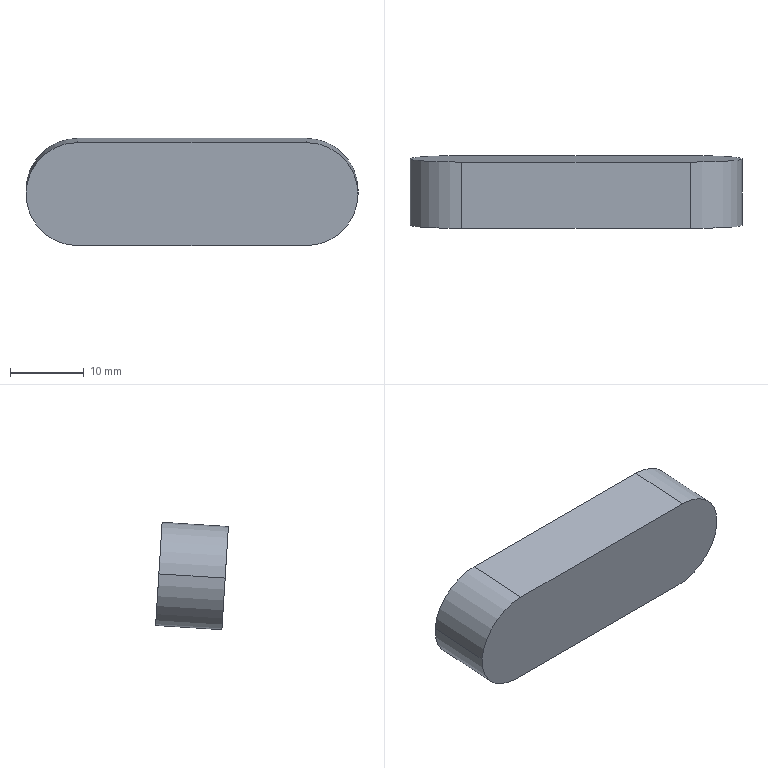Part | STEP file | Boss-Extrude 1-5 | 1 solid | 8 faces | box 45 x 9.869 x 14.542 mm | volume 5291 mm3 | cylinder 4 | plane 4 | commonest cylinder face diameters 14 x4
STEP:
#1=CARTESIAN_POINT('',(-140.476,-508.763,2440.556));
#2=VERTEX_POINT('',#1);
#3=CARTESIAN_POINT('',(-133.476,-509.206,2447.542));
#4=VERTEX_POINT('',#3);
#5=CARTESIAN_POINT('',(-133.476,-508.763,2440.556));
#6=DIRECTION('',(0.,0.998,0.06338));
#7=DIRECTION('',(-1.,0.,0.));
#8=AXIS2_PLACEMENT_3D('',#5,#6,#7);
#9=CIRCLE('',#8,7.);
#10=EDGE_CURVE('',#2,#4,#9,.T.);
#11=ORIENTED_EDGE('',*,*,#10,.F.);
#12=CARTESIAN_POINT('',(-140.476,-517.745,2439.986));
#13=VERTEX_POINT('',#12);
#14=CARTESIAN_POINT('',(-140.476,-508.763,2440.556));
#15=DIRECTION('',(0.,-0.998,-0.06338));
#16=VECTOR('',#15,1000.);
#17=LINE('',#14,#16);
#18=EDGE_CURVE('',#2,#13,#17,.T.);
#19=ORIENTED_EDGE('',*,*,#18,.T.);
#20=CARTESIAN_POINT('',(-133.476,-518.188,2446.972));
#21=VERTEX_POINT('',#20);
#22=CARTESIAN_POINT('',(-133.476,-517.745,2439.986));
#23=DIRECTION('',(0.,0.998,0.06338));
#24=DIRECTION('',(-1.,0.,0.));
#25=AXIS2_PLACEMENT_3D('',#22,#23,#24);
#26=CIRCLE('',#25,7.);
#27=EDGE_CURVE('',#13,#21,#26,.T.);
#28=ORIENTED_EDGE('',*,*,#27,.T.);
#29=CARTESIAN_POINT('',(-133.476,-509.206,2447.542));
#30=DIRECTION('',(0.,-0.998,-0.06338));
#31=VECTOR('',#30,1000.);
#32=LINE('',#29,#31);
#33=EDGE_CURVE('',#4,#21,#32,.T.);
#34=ORIENTED_EDGE('',*,*,#33,.F.);
#35=EDGE_LOOP('',(#11,#19,#28,#34));
#36=FACE_OUTER_BOUND('',#35,.T.);
#37=CARTESIAN_POINT('',(-133.476,-508.763,2440.556));
#38=DIRECTION('',(0.,-0.998,-0.06338));
#39=DIRECTION('',(-1.,0.,0.));
#40=AXIS2_PLACEMENT_3D('',#37,#38,#39);
#41=CYLINDRICAL_SURFACE('',#40,7.);
#42=ADVANCED_FACE('',(#36),#41,.T.);
#43=CARTESIAN_POINT('',(-95.476,-508.763,2440.556));
#44=VERTEX_POINT('',#43);
#45=CARTESIAN_POINT('',(-102.476,-508.319,2433.57));
#46=VERTEX_POINT('',#45);
#47=CARTESIAN_POINT('',(-102.476,-508.763,2440.556));
#48=DIRECTION('',(0.,0.998,0.06338));
#49=DIRECTION('',(-1.,0.,0.));
#50=AXIS2_PLACEMENT_3D('',#47,#48,#49);
#51=CIRCLE('',#50,7.);
#52=EDGE_CURVE('',#44,#46,#51,.T.);
#53=ORIENTED_EDGE('',*,*,#52,.F.);
#54=CARTESIAN_POINT('',(-95.476,-517.745,2439.986));
#55=VERTEX_POINT('',#54);
#56=CARTESIAN_POINT('',(-95.476,-508.763,2440.556));
#57=DIRECTION('',(0.,-0.998,-0.06338));
#58=VECTOR('',#57,1000.);
#59=LINE('',#56,#58);
#60=EDGE_CURVE('',#44,#55,#59,.T.);
#61=ORIENTED_EDGE('',*,*,#60,.T.);
#62=CARTESIAN_POINT('',(-102.476,-517.301,2433.));
#63=VERTEX_POINT('',#62);
#64=CARTESIAN_POINT('',(-102.476,-517.745,2439.986));
#65=DIRECTION('',(0.,0.998,0.06338));
#66=DIRECTION('',(-1.,0.,0.));
#67=AXIS2_PLACEMENT_3D('',#64,#65,#66);
#68=CIRCLE('',#67,7.);
#69=EDGE_CURVE('',#55,#63,#68,.T.);
#70=ORIENTED_EDGE('',*,*,#69,.T.);
#71=CARTESIAN_POINT('',(-102.476,-508.319,2433.57));
#72=DIRECTION('',(0.,-0.998,-0.06338));
#73=VECTOR('',#72,1000.);
#74=LINE('',#71,#73);
#75=EDGE_CURVE('',#46,#63,#74,.T.);
#76=ORIENTED_EDGE('',*,*,#75,.F.);
#77=EDGE_LOOP('',(#53,#61,#70,#76));
#78=FACE_OUTER_BOUND('',#77,.T.);
#79=CARTESIAN_POINT('',(-102.476,-508.763,2440.556));
#80=DIRECTION('',(0.,-0.998,-0.06338));
#81=DIRECTION('',(-1.,0.,0.));
#82=AXIS2_PLACEMENT_3D('',#79,#80,#81);
#83=CYLINDRICAL_SURFACE('',#82,7.);
#84=ADVANCED_FACE('',(#78),#83,.T.);
#85=ORIENTED_EDGE('',*,*,#60,.F.);
#86=CARTESIAN_POINT('',(-102.476,-509.206,2447.542));
#87=VERTEX_POINT('',#86);
#88=CARTESIAN_POINT('',(-102.476,-508.763,2440.556));
#89=DIRECTION('',(0.,0.998,0.06338));
#90=DIRECTION('',(-1.,0.,0.));
#91=AXIS2_PLACEMENT_3D('',#88,#89,#90);
#92=CIRCLE('',#91,7.);
#93=EDGE_CURVE('',#87,#44,#92,.T.);
#94=ORIENTED_EDGE('',*,*,#93,.F.);
#95=CARTESIAN_POINT('',(-102.476,-518.188,2446.972));
#96=VERTEX_POINT('',#95);
#97=CARTESIAN_POINT('',(-102.476,-509.206,2447.542));
#98=DIRECTION('',(0.,-0.998,-0.06338));
#99=VECTOR('',#98,1000.);
#100=LINE('',#97,#99);
#101=EDGE_CURVE('',#87,#96,#100,.T.);
#102=ORIENTED_EDGE('',*,*,#101,.T.);
#103=CARTESIAN_POINT('',(-102.476,-517.745,2439.986));
#104=DIRECTION('',(0.,0.998,0.06338));
#105=DIRECTION('',(-1.,0.,0.));
#106=AXIS2_PLACEMENT_3D('',#103,#104,#105);
#107=CIRCLE('',#106,7.);
#108=EDGE_CURVE('',#96,#55,#107,.T.);
#109=ORIENTED_EDGE('',*,*,#108,.T.);
#110=EDGE_LOOP('',(#85,#94,#102,#109));
#111=FACE_OUTER_BOUND('',#110,.T.);
#112=CARTESIAN_POINT('',(-102.476,-508.763,2440.556));
#113=DIRECTION('',(0.,-0.998,-0.06338));
#114=DIRECTION('',(-1.,0.,0.));
#115=AXIS2_PLACEMENT_3D('',#112,#113,#114);
#116=CYLINDRICAL_SURFACE('',#115,7.);
#117=ADVANCED_FACE('',(#111),#116,.T.);
#118=CARTESIAN_POINT('',(-133.476,-517.301,2433.));
#119=VERTEX_POINT('',#118);
#120=CARTESIAN_POINT('',(-102.476,-517.301,2433.));
#121=DIRECTION('',(-1.,0.,0.));
#122=VECTOR('',#121,1000.);
#123=LINE('',#120,#122);
#124=EDGE_CURVE('',#63,#119,#123,.T.);
#125=ORIENTED_EDGE('',*,*,#124,.T.);
#126=CARTESIAN_POINT('',(-133.476,-508.319,2433.57));
#127=VERTEX_POINT('',#126);
#128=CARTESIAN_POINT('',(-133.476,-508.319,2433.57));
#129=DIRECTION('',(0.,-0.998,-0.06338));
#130=VECTOR('',#129,1000.);
#131=LINE('',#128,#130);
#132=EDGE_CURVE('',#127,#119,#131,.T.);
#133=ORIENTED_EDGE('',*,*,#132,.F.);
#134=CARTESIAN_POINT('',(-102.476,-508.319,2433.57));
#135=DIRECTION('',(-1.,0.,0.));
#136=VECTOR('',#135,1000.);
#137=LINE('',#134,#136);
#138=EDGE_CURVE('',#46,#127,#137,.T.);
#139=ORIENTED_EDGE('',*,*,#138,.F.);
#140=ORIENTED_EDGE('',*,*,#75,.T.);
#141=EDGE_LOOP('',(#125,#133,#139,#140));
#142=FACE_OUTER_BOUND('',#141,.T.);
#143=CARTESIAN_POINT('',(-102.476,-508.319,2433.57));
#144=DIRECTION('',(0.,-0.06338,0.998));
#145=DIRECTION('',(-1.,0.,0.));
#146=AXIS2_PLACEMENT_3D('',#143,#144,#145);
#147=PLANE('',#146);
#148=ADVANCED_FACE('',(#142),#147,.F.);
#149=ORIENTED_EDGE('',*,*,#18,.F.);
#150=CARTESIAN_POINT('',(-133.476,-508.763,2440.556));
#151=DIRECTION('',(0.,0.998,0.06338));
#152=DIRECTION('',(-1.,0.,0.));
#153=AXIS2_PLACEMENT_3D('',#150,#151,#152);
#154=CIRCLE('',#153,7.);
#155=EDGE_CURVE('',#127,#2,#154,.T.);
#156=ORIENTED_EDGE('',*,*,#155,.F.);
#157=ORIENTED_EDGE('',*,*,#132,.T.);
#158=CARTESIAN_POINT('',(-133.476,-517.745,2439.986));
#159=DIRECTION('',(0.,0.998,0.06338));
#160=DIRECTION('',(-1.,0.,0.));
#161=AXIS2_PLACEMENT_3D('',#158,#159,#160);
#162=CIRCLE('',#161,7.);
#163=EDGE_CURVE('',#119,#13,#162,.T.);
#164=ORIENTED_EDGE('',*,*,#163,.T.);
#165=EDGE_LOOP('',(#149,#156,#157,#164));
#166=FACE_OUTER_BOUND('',#165,.T.);
#167=CARTESIAN_POINT('',(-133.476,-508.763,2440.556));
#168=DIRECTION('',(0.,-0.998,-0.06338));
#169=DIRECTION('',(-1.,0.,0.));
#170=AXIS2_PLACEMENT_3D('',#167,#168,#169);
#171=CYLINDRICAL_SURFACE('',#170,7.);
#172=ADVANCED_FACE('',(#166),#171,.T.);
#173=CARTESIAN_POINT('',(-102.476,-518.188,2446.972));
#174=DIRECTION('',(1.,0.,0.));
#175=VECTOR('',#174,1000.);
#176=LINE('',#173,#175);
#177=EDGE_CURVE('',#21,#96,#176,.T.);
#178=ORIENTED_EDGE('',*,*,#177,.T.);
#179=ORIENTED_EDGE('',*,*,#101,.F.);
#180=CARTESIAN_POINT('',(-102.476,-509.206,2447.542));
#181=DIRECTION('',(1.,0.,0.));
#182=VECTOR('',#181,1000.);
#183=LINE('',#180,#182);
#184=EDGE_CURVE('',#4,#87,#183,.T.);
#185=ORIENTED_EDGE('',*,*,#184,.F.);
#186=ORIENTED_EDGE('',*,*,#33,.T.);
#187=EDGE_LOOP('',(#178,#179,#185,#186));
#188=FACE_OUTER_BOUND('',#187,.T.);
#189=CARTESIAN_POINT('',(-102.476,-509.206,2447.542));
#190=DIRECTION('',(0.,0.06338,-0.998));
#191=DIRECTION('',(1.,0.,0.));
#192=AXIS2_PLACEMENT_3D('',#189,#190,#191);
#193=PLANE('',#192);
#194=ADVANCED_FACE('',(#188),#193,.F.);
#195=ORIENTED_EDGE('',*,*,#93,.T.);
#196=ORIENTED_EDGE('',*,*,#52,.T.);
#197=ORIENTED_EDGE('',*,*,#138,.T.);
#198=ORIENTED_EDGE('',*,*,#155,.T.);
#199=ORIENTED_EDGE('',*,*,#10,.T.);
#200=ORIENTED_EDGE('',*,*,#184,.T.);
#201=EDGE_LOOP('',(#195,#196,#197,#198,#199,#200));
#202=FACE_OUTER_BOUND('',#201,.T.);
#203=CARTESIAN_POINT('',(-102.476,-508.763,2440.556));
#204=DIRECTION('',(0.,0.998,0.06338));
#205=DIRECTION('',(1.,0.,0.));
#206=AXIS2_PLACEMENT_3D('',#203,#204,#205);
#207=PLANE('',#206);
#208=ADVANCED_FACE('',(#202),#207,.T.);
#209=ORIENTED_EDGE('',*,*,#108,.F.);
#210=ORIENTED_EDGE('',*,*,#177,.F.);
#211=ORIENTED_EDGE('',*,*,#27,.F.);
#212=ORIENTED_EDGE('',*,*,#163,.F.);
#213=ORIENTED_EDGE('',*,*,#124,.F.);
#214=ORIENTED_EDGE('',*,*,#69,.F.);
#215=EDGE_LOOP('',(#209,#210,#211,#212,#213,#214));
#216=FACE_OUTER_BOUND('',#215,.T.);
#217=CARTESIAN_POINT('',(-102.476,-517.745,2439.986));
#218=DIRECTION('',(0.,0.998,0.06338));
#219=DIRECTION('',(1.,0.,0.));
#220=AXIS2_PLACEMENT_3D('',#217,#218,#219);
#221=PLANE('',#220);
#222=ADVANCED_FACE('',(#216),#221,.F.);
#223=CLOSED_SHELL('',(#42,#84,#117,#148,#172,#194,#208,#222));
#224=MANIFOLD_SOLID_BREP('',#223);
#225=CARTESIAN_POINT('',(0.,0.,0.));
#226=DIRECTION('',(0.,0.,1.));
#227=DIRECTION('',(1.,0.,0.));
#228=AXIS2_PLACEMENT_3D('',#225,#226,#227);
#229=(LENGTH_UNIT()NAMED_UNIT(*)SI_UNIT(.MILLI.,.METRE.));
#230=UNCERTAINTY_MEASURE_WITH_UNIT(LENGTH_MEASURE(0.00001),#229,'','');
#231=(NAMED_UNIT(*)PLANE_ANGLE_UNIT()SI_UNIT($,.RADIAN.));
#232=(NAMED_UNIT(*)SI_UNIT($,.STERADIAN.)SOLID_ANGLE_UNIT());
#233=(GEOMETRIC_REPRESENTATION_CONTEXT(3)GLOBAL_UNCERTAINTY_ASSIGNED_CONTEXT((#230))GLOBAL_UNIT_ASSIGNED_CONTEXT((#229,#231,#232))REPRESENTATION_CONTEXT('',''));
#234=ADVANCED_BREP_SHAPE_REPRESENTATION('',(#224,#228),#233);